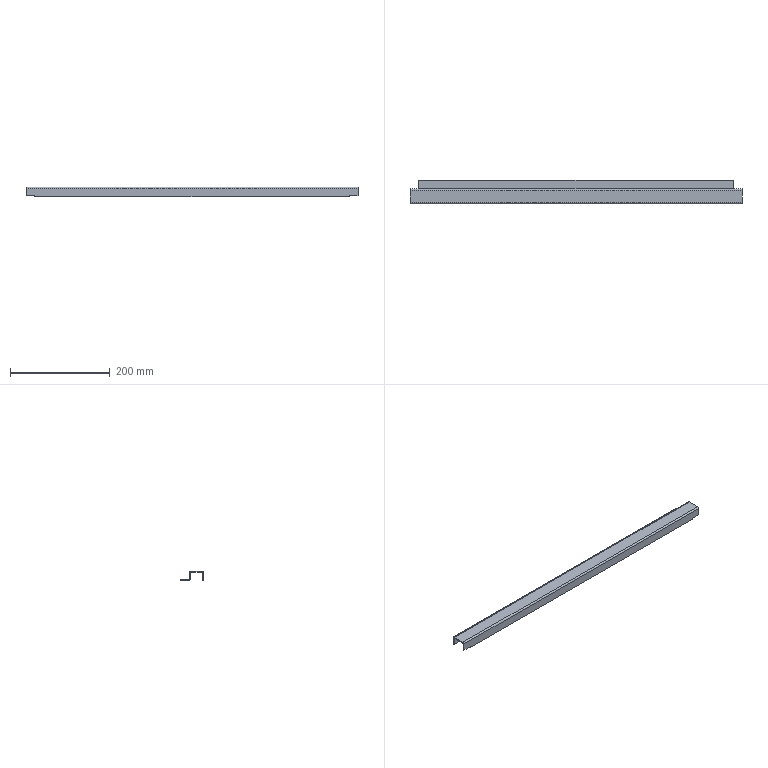Part | SolidWorks | features BaseBody 1 | 1 solid | 44 faces | box 667 x 48 x 20 mm | volume 107090 mm3 | plane 38 | cylinder 6 | commonest cylinder face diameters 2 x3 6 x3
STEP:
#1=CARTESIAN_POINT('',(-315.5,-13.,-18.));
#2=VERTEX_POINT('',#1);
#3=CARTESIAN_POINT('',(-315.5,-13.,-20.));
#4=VERTEX_POINT('',#3);
#5=CARTESIAN_POINT('',(-315.5,-13.,0.));
#6=DIRECTION('',(0.,0.,-1.));
#7=VECTOR('',#6,1000.);
#8=LINE('',#5,#7);
#9=EDGE_CURVE('',#2,#4,#8,.T.);
#10=ORIENTED_EDGE('',*,*,#9,.T.);
#11=CARTESIAN_POINT('',(-315.5,-15.,-20.));
#12=VERTEX_POINT('',#11);
#13=CARTESIAN_POINT('',(-315.5,33.,-20.));
#14=DIRECTION('',(0.,-1.,0.));
#15=VECTOR('',#14,1000.);
#16=LINE('',#13,#15);
#17=EDGE_CURVE('',#4,#12,#16,.T.);
#18=ORIENTED_EDGE('',*,*,#17,.T.);
#19=CARTESIAN_POINT('',(-315.5,-15.,-18.));
#20=VERTEX_POINT('',#19);
#21=CARTESIAN_POINT('',(-315.5,-15.,-20.));
#22=DIRECTION('',(0.,0.,1.));
#23=VECTOR('',#22,1000.);
#24=LINE('',#21,#23);
#25=EDGE_CURVE('',#12,#20,#24,.T.);
#26=ORIENTED_EDGE('',*,*,#25,.T.);
#27=CARTESIAN_POINT('',(-315.5,33.,-18.));
#28=DIRECTION('',(0.,-1.,0.));
#29=VECTOR('',#28,1000.);
#30=LINE('',#27,#29);
#31=EDGE_CURVE('',#2,#20,#30,.T.);
#32=ORIENTED_EDGE('',*,*,#31,.F.);
#33=EDGE_LOOP('',(#10,#18,#26,#32));
#34=FACE_OUTER_BOUND('',#33,.T.);
#35=CARTESIAN_POINT('',(-315.5,33.,-20.));
#36=DIRECTION('',(1.,0.,0.));
#37=DIRECTION('',(0.,1.,0.));
#38=AXIS2_PLACEMENT_3D('',#35,#36,#37);
#39=PLANE('',#38);
#40=ADVANCED_FACE('',(#34),#39,.F.);
#41=CARTESIAN_POINT('',(-333.5,-13.,-18.));
#42=VERTEX_POINT('',#41);
#43=CARTESIAN_POINT('',(0.,-13.,-18.));
#44=DIRECTION('',(1.,0.,0.));
#45=VECTOR('',#44,1000.);
#46=LINE('',#43,#45);
#47=EDGE_CURVE('',#42,#2,#46,.T.);
#48=ORIENTED_EDGE('',*,*,#47,.T.);
#49=ORIENTED_EDGE('',*,*,#31,.T.);
#50=CARTESIAN_POINT('',(-333.5,-15.,-18.));
#51=VERTEX_POINT('',#50);
#52=CARTESIAN_POINT('',(-333.5,-15.,-18.));
#53=DIRECTION('',(-1.,0.,0.));
#54=VECTOR('',#53,1000.);
#55=LINE('',#52,#54);
#56=EDGE_CURVE('',#20,#51,#55,.T.);
#57=ORIENTED_EDGE('',*,*,#56,.T.);
#58=CARTESIAN_POINT('',(-333.5,33.,-18.));
#59=DIRECTION('',(0.,-1.,0.));
#60=VECTOR('',#59,1000.);
#61=LINE('',#58,#60);
#62=EDGE_CURVE('',#42,#51,#61,.T.);
#63=ORIENTED_EDGE('',*,*,#62,.F.);
#64=EDGE_LOOP('',(#48,#49,#57,#63));
#65=FACE_OUTER_BOUND('',#64,.T.);
#66=CARTESIAN_POINT('',(-333.5,33.,-18.));
#67=DIRECTION('',(0.,0.,1.));
#68=DIRECTION('',(0.,-1.,0.));
#69=AXIS2_PLACEMENT_3D('',#66,#67,#68);
#70=PLANE('',#69);
#71=ADVANCED_FACE('',(#65),#70,.F.);
#72=CARTESIAN_POINT('',(315.5,-13.,-20.));
#73=VERTEX_POINT('',#72);
#74=CARTESIAN_POINT('',(315.5,-13.,-18.));
#75=VERTEX_POINT('',#74);
#76=CARTESIAN_POINT('',(315.5,-13.,0.));
#77=DIRECTION('',(0.,0.,1.));
#78=VECTOR('',#77,1000.);
#79=LINE('',#76,#78);
#80=EDGE_CURVE('',#73,#75,#79,.T.);
#81=ORIENTED_EDGE('',*,*,#80,.T.);
#82=CARTESIAN_POINT('',(315.5,-15.,-18.));
#83=VERTEX_POINT('',#82);
#84=CARTESIAN_POINT('',(315.5,33.,-18.));
#85=DIRECTION('',(0.,-1.,0.));
#86=VECTOR('',#85,1000.);
#87=LINE('',#84,#86);
#88=EDGE_CURVE('',#75,#83,#87,.T.);
#89=ORIENTED_EDGE('',*,*,#88,.T.);
#90=CARTESIAN_POINT('',(315.5,-15.,-20.));
#91=VERTEX_POINT('',#90);
#92=CARTESIAN_POINT('',(315.5,-15.,-20.));
#93=DIRECTION('',(0.,0.,-1.));
#94=VECTOR('',#93,1000.);
#95=LINE('',#92,#94);
#96=EDGE_CURVE('',#83,#91,#95,.T.);
#97=ORIENTED_EDGE('',*,*,#96,.T.);
#98=CARTESIAN_POINT('',(315.5,33.,-20.));
#99=DIRECTION('',(0.,-1.,0.));
#100=VECTOR('',#99,1000.);
#101=LINE('',#98,#100);
#102=EDGE_CURVE('',#73,#91,#101,.T.);
#103=ORIENTED_EDGE('',*,*,#102,.F.);
#104=EDGE_LOOP('',(#81,#89,#97,#103));
#105=FACE_OUTER_BOUND('',#104,.T.);
#106=CARTESIAN_POINT('',(315.5,33.,-20.));
#107=DIRECTION('',(-1.,0.,0.));
#108=DIRECTION('',(0.,1.,0.));
#109=AXIS2_PLACEMENT_3D('',#106,#107,#108);
#110=PLANE('',#109);
#111=ADVANCED_FACE('',(#105),#110,.F.);
#112=CARTESIAN_POINT('',(333.5,-13.,-18.));
#113=VERTEX_POINT('',#112);
#114=CARTESIAN_POINT('',(0.,-13.,-18.));
#115=DIRECTION('',(1.,0.,0.));
#116=VECTOR('',#115,1000.);
#117=LINE('',#114,#116);
#118=EDGE_CURVE('',#75,#113,#117,.T.);
#119=ORIENTED_EDGE('',*,*,#118,.T.);
#120=CARTESIAN_POINT('',(333.5,-15.,-18.));
#121=VERTEX_POINT('',#120);
#122=CARTESIAN_POINT('',(333.5,33.,-18.));
#123=DIRECTION('',(0.,-1.,0.));
#124=VECTOR('',#123,1000.);
#125=LINE('',#122,#124);
#126=EDGE_CURVE('',#113,#121,#125,.T.);
#127=ORIENTED_EDGE('',*,*,#126,.T.);
#128=CARTESIAN_POINT('',(333.5,-15.,-18.));
#129=DIRECTION('',(-1.,0.,0.));
#130=VECTOR('',#129,1000.);
#131=LINE('',#128,#130);
#132=EDGE_CURVE('',#121,#83,#131,.T.);
#133=ORIENTED_EDGE('',*,*,#132,.T.);
#134=ORIENTED_EDGE('',*,*,#88,.F.);
#135=EDGE_LOOP('',(#119,#127,#133,#134));
#136=FACE_OUTER_BOUND('',#135,.T.);
#137=CARTESIAN_POINT('',(333.5,33.,-18.));
#138=DIRECTION('',(0.,0.,1.));
#139=DIRECTION('',(0.,-1.,0.));
#140=AXIS2_PLACEMENT_3D('',#137,#138,#139);
#141=PLANE('',#140);
#142=ADVANCED_FACE('',(#136),#141,.F.);
#143=CARTESIAN_POINT('',(-333.5,15.,-18.));
#144=VERTEX_POINT('',#143);
#145=CARTESIAN_POINT('',(-316.5,15.,-18.));
#146=VERTEX_POINT('',#145);
#147=CARTESIAN_POINT('',(0.,15.,-18.));
#148=DIRECTION('',(1.,0.,0.));
#149=VECTOR('',#148,1000.);
#150=LINE('',#147,#149);
#151=EDGE_CURVE('',#144,#146,#150,.T.);
#152=ORIENTED_EDGE('',*,*,#151,.T.);
#153=CARTESIAN_POINT('',(-316.5,13.,-18.));
#154=VERTEX_POINT('',#153);
#155=CARTESIAN_POINT('',(-316.5,15.,-18.));
#156=DIRECTION('',(0.,-1.,0.));
#157=VECTOR('',#156,1000.);
#158=LINE('',#155,#157);
#159=EDGE_CURVE('',#146,#154,#158,.T.);
#160=ORIENTED_EDGE('',*,*,#159,.T.);
#161=CARTESIAN_POINT('',(-333.5,13.,-18.));
#162=VERTEX_POINT('',#161);
#163=CARTESIAN_POINT('',(0.,13.,-18.));
#164=DIRECTION('',(1.,0.,0.));
#165=VECTOR('',#164,1000.);
#166=LINE('',#163,#165);
#167=EDGE_CURVE('',#162,#154,#166,.T.);
#168=ORIENTED_EDGE('',*,*,#167,.F.);
#169=CARTESIAN_POINT('',(-333.5,33.,-18.));
#170=DIRECTION('',(0.,-1.,0.));
#171=VECTOR('',#170,1000.);
#172=LINE('',#169,#171);
#173=EDGE_CURVE('',#144,#162,#172,.T.);
#174=ORIENTED_EDGE('',*,*,#173,.F.);
#175=EDGE_LOOP('',(#152,#160,#168,#174));
#176=FACE_OUTER_BOUND('',#175,.T.);
#177=CARTESIAN_POINT('',(-333.5,33.,-18.));
#178=DIRECTION('',(0.,0.,1.));
#179=DIRECTION('',(0.,-1.,0.));
#180=AXIS2_PLACEMENT_3D('',#177,#178,#179);
#181=PLANE('',#180);
#182=ADVANCED_FACE('',(#176),#181,.F.);
#183=CARTESIAN_POINT('',(316.5,15.,-18.));
#184=VERTEX_POINT('',#183);
#185=CARTESIAN_POINT('',(333.5,15.,-18.));
#186=VERTEX_POINT('',#185);
#187=CARTESIAN_POINT('',(0.,15.,-18.));
#188=DIRECTION('',(1.,0.,0.));
#189=VECTOR('',#188,1000.);
#190=LINE('',#187,#189);
#191=EDGE_CURVE('',#184,#186,#190,.T.);
#192=ORIENTED_EDGE('',*,*,#191,.T.);
#193=CARTESIAN_POINT('',(333.5,13.,-18.));
#194=VERTEX_POINT('',#193);
#195=CARTESIAN_POINT('',(333.5,33.,-18.));
#196=DIRECTION('',(0.,-1.,0.));
#197=VECTOR('',#196,1000.);
#198=LINE('',#195,#197);
#199=EDGE_CURVE('',#186,#194,#198,.T.);
#200=ORIENTED_EDGE('',*,*,#199,.T.);
#201=CARTESIAN_POINT('',(316.5,13.,-18.));
#202=VERTEX_POINT('',#201);
#203=CARTESIAN_POINT('',(0.,13.,-18.));
#204=DIRECTION('',(1.,0.,0.));
#205=VECTOR('',#204,1000.);
#206=LINE('',#203,#205);
#207=EDGE_CURVE('',#202,#194,#206,.T.);
#208=ORIENTED_EDGE('',*,*,#207,.F.);
#209=CARTESIAN_POINT('',(316.5,15.,-18.));
#210=DIRECTION('',(0.,1.,0.));
#211=VECTOR('',#210,1000.);
#212=LINE('',#209,#211);
#213=EDGE_CURVE('',#202,#184,#212,.T.);
#214=ORIENTED_EDGE('',*,*,#213,.T.);
#215=EDGE_LOOP('',(#192,#200,#208,#214));
#216=FACE_OUTER_BOUND('',#215,.T.);
#217=CARTESIAN_POINT('',(333.5,33.,-18.));
#218=DIRECTION('',(0.,0.,1.));
#219=DIRECTION('',(0.,-1.,0.));
#220=AXIS2_PLACEMENT_3D('',#217,#218,#219);
#221=PLANE('',#220);
#222=ADVANCED_FACE('',(#216),#221,.F.);
#223=CARTESIAN_POINT('',(315.5,33.,-18.));
#224=VERTEX_POINT('',#223);
#225=CARTESIAN_POINT('',(-315.5,33.,-18.));
#226=VERTEX_POINT('',#225);
#227=CARTESIAN_POINT('',(0.,33.,-18.));
#228=DIRECTION('',(-1.,0.,0.));
#229=VECTOR('',#228,1000.);
#230=LINE('',#227,#229);
#231=EDGE_CURVE('',#224,#226,#230,.T.);
#232=ORIENTED_EDGE('',*,*,#231,.F.);
#233=CARTESIAN_POINT('',(315.5,33.,-20.));
#234=VERTEX_POINT('',#233);
#235=CARTESIAN_POINT('',(315.5,33.,-20.));
#236=DIRECTION('',(0.,0.,1.));
#237=VECTOR('',#236,1000.);
#238=LINE('',#235,#237);
#239=EDGE_CURVE('',#234,#224,#238,.T.);
#240=ORIENTED_EDGE('',*,*,#239,.F.);
#241=CARTESIAN_POINT('',(-315.5,33.,-20.));
#242=VERTEX_POINT('',#241);
#243=CARTESIAN_POINT('',(-315.5,33.,-20.));
#244=DIRECTION('',(-1.,0.,0.));
#245=VECTOR('',#244,1000.);
#246=LINE('',#243,#245);
#247=EDGE_CURVE('',#234,#242,#246,.T.);
#248=ORIENTED_EDGE('',*,*,#247,.T.);
#249=CARTESIAN_POINT('',(-315.5,33.,-20.));
#250=DIRECTION('',(0.,0.,1.));
#251=VECTOR('',#250,1000.);
#252=LINE('',#249,#251);
#253=EDGE_CURVE('',#242,#226,#252,.T.);
#254=ORIENTED_EDGE('',*,*,#253,.T.);
#255=EDGE_LOOP('',(#232,#240,#248,#254));
#256=FACE_OUTER_BOUND('',#255,.T.);
#257=CARTESIAN_POINT('',(-315.5,33.,-20.));
#258=DIRECTION('',(0.,1.,0.));
#259=DIRECTION('',(1.,0.,0.));
#260=AXIS2_PLACEMENT_3D('',#257,#258,#259);
#261=PLANE('',#260);
#262=ADVANCED_FACE('',(#256),#261,.T.);
#263=CARTESIAN_POINT('',(315.5,16.,-18.));
#264=VERTEX_POINT('',#263);
#265=CARTESIAN_POINT('',(-315.5,16.,-18.));
#266=VERTEX_POINT('',#265);
#267=CARTESIAN_POINT('',(315.5,16.,-18.));
#268=DIRECTION('',(-1.,0.,0.));
#269=VECTOR('',#268,1000.);
#270=LINE('',#267,#269);
#271=EDGE_CURVE('',#264,#266,#270,.T.);
#272=ORIENTED_EDGE('',*,*,#271,.F.);
#273=CARTESIAN_POINT('',(315.5,0.,-18.));
#274=DIRECTION('',(0.,1.,0.));
#275=VECTOR('',#274,1000.);
#276=LINE('',#273,#275);
#277=EDGE_CURVE('',#264,#224,#276,.T.);
#278=ORIENTED_EDGE('',*,*,#277,.T.);
#279=ORIENTED_EDGE('',*,*,#231,.T.);
#280=CARTESIAN_POINT('',(-315.5,0.,-18.));
#281=DIRECTION('',(0.,-1.,0.));
#282=VECTOR('',#281,1000.);
#283=LINE('',#280,#282);
#284=EDGE_CURVE('',#226,#266,#283,.T.);
#285=ORIENTED_EDGE('',*,*,#284,.T.);
#286=EDGE_LOOP('',(#272,#278,#279,#285));
#287=FACE_OUTER_BOUND('',#286,.T.);
#288=CARTESIAN_POINT('',(0.,0.,-18.));
#289=DIRECTION('',(0.,0.,-1.));
#290=DIRECTION('',(0.,-1.,0.));
#291=AXIS2_PLACEMENT_3D('',#288,#289,#290);
#292=PLANE('',#291);
#293=ADVANCED_FACE('',(#287),#292,.F.);
#294=CARTESIAN_POINT('',(315.5,16.,-20.));
#295=VERTEX_POINT('',#294);
#296=CARTESIAN_POINT('',(315.5,15.,-20.));
#297=DIRECTION('',(0.,1.,0.));
#298=VECTOR('',#297,1000.);
#299=LINE('',#296,#298);
#300=EDGE_CURVE('',#295,#234,#299,.T.);
#301=ORIENTED_EDGE('',*,*,#300,.F.);
#302=CARTESIAN_POINT('',(-315.5,16.,-20.));
#303=VERTEX_POINT('',#302);
#304=CARTESIAN_POINT('',(0.,16.,-20.));
#305=DIRECTION('',(-1.,0.,0.));
#306=VECTOR('',#305,1000.);
#307=LINE('',#304,#306);
#308=EDGE_CURVE('',#295,#303,#307,.T.);
#309=ORIENTED_EDGE('',*,*,#308,.T.);
#310=CARTESIAN_POINT('',(-315.5,15.,-20.));
#311=DIRECTION('',(0.,-1.,0.));
#312=VECTOR('',#311,1000.);
#313=LINE('',#310,#312);
#314=EDGE_CURVE('',#242,#303,#313,.T.);
#315=ORIENTED_EDGE('',*,*,#314,.F.);
#316=ORIENTED_EDGE('',*,*,#247,.F.);
#317=EDGE_LOOP('',(#301,#309,#315,#316));
#318=FACE_OUTER_BOUND('',#317,.T.);
#319=CARTESIAN_POINT('',(0.,0.,-20.));
#320=DIRECTION('',(0.,0.,-1.));
#321=DIRECTION('',(0.,-1.,0.));
#322=AXIS2_PLACEMENT_3D('',#319,#320,#321);
#323=PLANE('',#322);
#324=ADVANCED_FACE('',(#318),#323,.T.);
#325=ORIENTED_EDGE('',*,*,#314,.T.);
#326=CARTESIAN_POINT('',(-315.5,16.,-18.));
#327=DIRECTION('',(0.,0.,-1.));
#328=VECTOR('',#327,1000.);
#329=LINE('',#326,#328);
#330=EDGE_CURVE('',#266,#303,#329,.T.);
#331=ORIENTED_EDGE('',*,*,#330,.F.);
#332=ORIENTED_EDGE('',*,*,#284,.F.);
#333=ORIENTED_EDGE('',*,*,#253,.F.);
#334=EDGE_LOOP('',(#325,#331,#332,#333));
#335=FACE_OUTER_BOUND('',#334,.T.);
#336=CARTESIAN_POINT('',(-315.5,15.,-20.));
#337=DIRECTION('',(-1.,0.,0.));
#338=DIRECTION('',(0.,0.,1.));
#339=AXIS2_PLACEMENT_3D('',#336,#337,#338);
#340=PLANE('',#339);
#341=ADVANCED_FACE('',(#335),#340,.T.);
#342=ORIENTED_EDGE('',*,*,#277,.F.);
#343=CARTESIAN_POINT('',(315.5,16.,-20.));
#344=DIRECTION('',(0.,0.,-1.));
#345=VECTOR('',#344,1000.);
#346=LINE('',#343,#345);
#347=EDGE_CURVE('',#264,#295,#346,.T.);
#348=ORIENTED_EDGE('',*,*,#347,.T.);
#349=ORIENTED_EDGE('',*,*,#300,.T.);
#350=ORIENTED_EDGE('',*,*,#239,.T.);
#351=EDGE_LOOP('',(#342,#348,#349,#350));
#352=FACE_OUTER_BOUND('',#351,.T.);
#353=CARTESIAN_POINT('',(315.5,15.,-20.));
#354=DIRECTION('',(1.,0.,0.));
#355=DIRECTION('',(0.,1.,0.));
#356=AXIS2_PLACEMENT_3D('',#353,#354,#355);
#357=PLANE('',#356);
#358=ADVANCED_FACE('',(#352),#357,.T.);
#359=CARTESIAN_POINT('',(-315.5,15.,-17.));
#360=VERTEX_POINT('',#359);
#361=CARTESIAN_POINT('',(315.5,15.,-17.));
#362=VERTEX_POINT('',#361);
#363=CARTESIAN_POINT('',(-315.5,15.,-17.));
#364=DIRECTION('',(1.,0.,0.));
#365=VECTOR('',#364,1000.);
#366=LINE('',#363,#365);
#367=EDGE_CURVE('',#360,#362,#366,.T.);
#368=ORIENTED_EDGE('',*,*,#367,.T.);
#369=CARTESIAN_POINT('',(315.5,16.,-17.));
#370=DIRECTION('',(1.,0.,0.));
#371=DIRECTION('',(0.,0.,1.));
#372=AXIS2_PLACEMENT_3D('',#369,#370,#371);
#373=CIRCLE('',#372,1.);
#374=EDGE_CURVE('',#362,#264,#373,.T.);
#375=ORIENTED_EDGE('',*,*,#374,.T.);
#376=ORIENTED_EDGE('',*,*,#271,.T.);
#377=CARTESIAN_POINT('',(-315.5,16.,-17.));
#378=DIRECTION('',(-1.,0.,0.));
#379=DIRECTION('',(0.,0.,1.));
#380=AXIS2_PLACEMENT_3D('',#377,#378,#379);
#381=CIRCLE('',#380,1.);
#382=EDGE_CURVE('',#266,#360,#381,.T.);
#383=ORIENTED_EDGE('',*,*,#382,.T.);
#384=EDGE_LOOP('',(#368,#375,#376,#383));
#385=FACE_OUTER_BOUND('',#384,.T.);
#386=CARTESIAN_POINT('',(-315.5,16.,-17.));
#387=DIRECTION('',(-1.,0.,0.));
#388=DIRECTION('',(0.,0.,-1.));
#389=AXIS2_PLACEMENT_3D('',#386,#387,#388);
#390=CYLINDRICAL_SURFACE('',#389,1.);
#391=ADVANCED_FACE('',(#385),#390,.F.);
#392=CARTESIAN_POINT('',(-315.5,13.,-17.));
#393=VERTEX_POINT('',#392);
#394=CARTESIAN_POINT('',(315.5,13.,-17.));
#395=VERTEX_POINT('',#394);
#396=CARTESIAN_POINT('',(-315.5,13.,-17.));
#397=DIRECTION('',(1.,0.,0.));
#398=VECTOR('',#397,1000.);
#399=LINE('',#396,#398);
#400=EDGE_CURVE('',#393,#395,#399,.T.);
#401=ORIENTED_EDGE('',*,*,#400,.F.);
#402=CARTESIAN_POINT('',(-315.5,13.172,-18.));
#403=VERTEX_POINT('',#402);
#404=CARTESIAN_POINT('',(-315.5,16.,-17.));
#405=DIRECTION('',(-1.,0.,0.));
#406=DIRECTION('',(0.,0.,1.));
#407=AXIS2_PLACEMENT_3D('',#404,#405,#406);
#408=CIRCLE('',#407,3.);
#409=EDGE_CURVE('',#403,#393,#408,.T.);
#410=ORIENTED_EDGE('',*,*,#409,.F.);
#411=CARTESIAN_POINT('',(-315.5,16.,-17.));
#412=DIRECTION('',(-1.,0.,0.));
#413=DIRECTION('',(0.,0.,1.));
#414=AXIS2_PLACEMENT_3D('',#411,#412,#413);
#415=CIRCLE('',#414,3.);
#416=EDGE_CURVE('',#303,#403,#415,.T.);
#417=ORIENTED_EDGE('',*,*,#416,.F.);
#418=ORIENTED_EDGE('',*,*,#308,.F.);
#419=CARTESIAN_POINT('',(315.5,13.172,-18.));
#420=VERTEX_POINT('',#419);
#421=CARTESIAN_POINT('',(315.5,16.,-17.));
#422=DIRECTION('',(1.,0.,0.));
#423=DIRECTION('',(0.,0.,1.));
#424=AXIS2_PLACEMENT_3D('',#421,#422,#423);
#425=CIRCLE('',#424,3.);
#426=EDGE_CURVE('',#420,#295,#425,.T.);
#427=ORIENTED_EDGE('',*,*,#426,.F.);
#428=CARTESIAN_POINT('',(315.5,16.,-17.));
#429=DIRECTION('',(1.,0.,0.));
#430=DIRECTION('',(0.,0.,1.));
#431=AXIS2_PLACEMENT_3D('',#428,#429,#430);
#432=CIRCLE('',#431,3.);
#433=EDGE_CURVE('',#395,#420,#432,.T.);
#434=ORIENTED_EDGE('',*,*,#433,.F.);
#435=EDGE_LOOP('',(#401,#410,#417,#418,#427,#434));
#436=FACE_OUTER_BOUND('',#435,.T.);
#437=CARTESIAN_POINT('',(-315.5,16.,-17.));
#438=DIRECTION('',(-1.,0.,0.));
#439=DIRECTION('',(0.,0.,-1.));
#440=AXIS2_PLACEMENT_3D('',#437,#438,#439);
#441=CYLINDRICAL_SURFACE('',#440,3.);
#442=ADVANCED_FACE('',(#436),#441,.T.);
#443=CARTESIAN_POINT('',(-315.5,16.,-18.));
#444=DIRECTION('',(0.,1.,0.));
#445=VECTOR('',#444,1000.);
#446=LINE('',#443,#445);
#447=EDGE_CURVE('',#403,#266,#446,.T.);
#448=ORIENTED_EDGE('',*,*,#447,.F.);
#449=ORIENTED_EDGE('',*,*,#409,.T.);
#450=CARTESIAN_POINT('',(-315.5,15.,-17.));
#451=DIRECTION('',(0.,-1.,0.));
#452=VECTOR('',#451,1000.);
#453=LINE('',#450,#452);
#454=EDGE_CURVE('',#360,#393,#453,.T.);
#455=ORIENTED_EDGE('',*,*,#454,.F.);
#456=ORIENTED_EDGE('',*,*,#382,.F.);
#457=EDGE_LOOP('',(#448,#449,#455,#456));
#458=FACE_OUTER_BOUND('',#457,.T.);
#459=CARTESIAN_POINT('',(-315.5,16.,-17.));
#460=DIRECTION('',(1.,0.,0.));
#461=DIRECTION('',(0.,1.,0.));
#462=AXIS2_PLACEMENT_3D('',#459,#460,#461);
#463=PLANE('',#462);
#464=ADVANCED_FACE('',(#458),#463,.F.);
#465=CARTESIAN_POINT('',(315.5,16.,-18.));
#466=DIRECTION('',(0.,-1.,0.));
#467=VECTOR('',#466,1000.);
#468=LINE('',#465,#467);
#469=EDGE_CURVE('',#264,#420,#468,.T.);
#470=ORIENTED_EDGE('',*,*,#469,.F.);
#471=ORIENTED_EDGE('',*,*,#374,.F.);
#472=CARTESIAN_POINT('',(315.5,15.,-17.));
#473=DIRECTION('',(0.,-1.,0.));
#474=VECTOR('',#473,1000.);
#475=LINE('',#472,#474);
#476=EDGE_CURVE('',#362,#395,#475,.T.);
#477=ORIENTED_EDGE('',*,*,#476,.T.);
#478=ORIENTED_EDGE('',*,*,#433,.T.);
#479=EDGE_LOOP('',(#470,#471,#477,#478));
#480=FACE_OUTER_BOUND('',#479,.T.);
#481=CARTESIAN_POINT('',(315.5,16.,-17.));
#482=DIRECTION('',(1.,0.,0.));
#483=DIRECTION('',(0.,1.,0.));
#484=AXIS2_PLACEMENT_3D('',#481,#482,#483);
#485=PLANE('',#484);
#486=ADVANCED_FACE('',(#480),#485,.T.);
#487=ORIENTED_EDGE('',*,*,#213,.F.);
#488=CARTESIAN_POINT('',(316.5,13.,-16.));
#489=VERTEX_POINT('',#488);
#490=CARTESIAN_POINT('',(316.5,13.,0.));
#491=DIRECTION('',(0.,0.,1.));
#492=VECTOR('',#491,1000.);
#493=LINE('',#490,#492);
#494=EDGE_CURVE('',#202,#489,#493,.T.);
#495=ORIENTED_EDGE('',*,*,#494,.T.);
#496=CARTESIAN_POINT('',(316.5,15.,-16.));
#497=VERTEX_POINT('',#496);
#498=CARTESIAN_POINT('',(316.5,15.,-16.));
#499=DIRECTION('',(0.,-1.,0.));
#500=VECTOR('',#499,1000.);
#501=LINE('',#498,#500);
#502=EDGE_CURVE('',#497,#489,#501,.T.);
#503=ORIENTED_EDGE('',*,*,#502,.F.);
#504=CARTESIAN_POINT('',(316.5,15.,-16.));
#505=DIRECTION('',(0.,0.,-1.));
#506=VECTOR('',#505,1000.);
#507=LINE('',#504,#506);
#508=EDGE_CURVE('',#497,#184,#507,.T.);
#509=ORIENTED_EDGE('',*,*,#508,.T.);
#510=EDGE_LOOP('',(#487,#495,#503,#509));
#511=FACE_OUTER_BOUND('',#510,.T.);
#512=CARTESIAN_POINT('',(316.5,15.,-16.));
#513=DIRECTION('',(-1.,0.,0.));
#514=DIRECTION('',(0.,0.,1.));
#515=AXIS2_PLACEMENT_3D('',#512,#513,#514);
#516=PLANE('',#515);
#517=ADVANCED_FACE('',(#511),#516,.T.);
#518=ORIENTED_EDGE('',*,*,#159,.F.);
#519=CARTESIAN_POINT('',(-316.5,15.,-16.));
#520=VERTEX_POINT('',#519);
#521=CARTESIAN_POINT('',(-316.5,15.,-20.));
#522=DIRECTION('',(0.,0.,1.));
#523=VECTOR('',#522,1000.);
#524=LINE('',#521,#523);
#525=EDGE_CURVE('',#146,#520,#524,.T.);
#526=ORIENTED_EDGE('',*,*,#525,.T.);
#527=CARTESIAN_POINT('',(-316.5,13.,-16.));
#528=VERTEX_POINT('',#527);
#529=CARTESIAN_POINT('',(-316.5,15.,-16.));
#530=DIRECTION('',(0.,-1.,0.));
#531=VECTOR('',#530,1000.);
#532=LINE('',#529,#531);
#533=EDGE_CURVE('',#520,#528,#532,.T.);
#534=ORIENTED_EDGE('',*,*,#533,.T.);
#535=CARTESIAN_POINT('',(-316.5,13.,0.));
#536=DIRECTION('',(0.,0.,-1.));
#537=VECTOR('',#536,1000.);
#538=LINE('',#535,#537);
#539=EDGE_CURVE('',#528,#154,#538,.T.);
#540=ORIENTED_EDGE('',*,*,#539,.T.);
#541=EDGE_LOOP('',(#518,#526,#534,#540));
#542=FACE_OUTER_BOUND('',#541,.T.);
#543=CARTESIAN_POINT('',(-316.5,15.,-20.));
#544=DIRECTION('',(1.,0.,0.));
#545=DIRECTION('',(0.,1.,0.));
#546=AXIS2_PLACEMENT_3D('',#543,#544,#545);
#547=PLANE('',#546);
#548=ADVANCED_FACE('',(#542),#547,.T.);
#549=ORIENTED_EDGE('',*,*,#502,.T.);
#550=CARTESIAN_POINT('',(315.5,13.,-16.));
#551=VERTEX_POINT('',#550);
#552=CARTESIAN_POINT('',(0.,13.,-16.));
#553=DIRECTION('',(-1.,0.,0.));
#554=VECTOR('',#553,1000.);
#555=LINE('',#552,#554);
#556=EDGE_CURVE('',#489,#551,#555,.T.);
#557=ORIENTED_EDGE('',*,*,#556,.T.);
#558=CARTESIAN_POINT('',(315.5,15.,-16.));
#559=VERTEX_POINT('',#558);
#560=CARTESIAN_POINT('',(315.5,15.,-16.));
#561=DIRECTION('',(0.,-1.,0.));
#562=VECTOR('',#561,1000.);
#563=LINE('',#560,#562);
#564=EDGE_CURVE('',#559,#551,#563,.T.);
#565=ORIENTED_EDGE('',*,*,#564,.F.);
#566=CARTESIAN_POINT('',(315.5,15.,-16.));
#567=DIRECTION('',(1.,0.,0.));
#568=VECTOR('',#567,1000.);
#569=LINE('',#566,#568);
#570=EDGE_CURVE('',#559,#497,#569,.T.);
#571=ORIENTED_EDGE('',*,*,#570,.T.);
#572=EDGE_LOOP('',(#549,#557,#565,#571));
#573=FACE_OUTER_BOUND('',#572,.T.);
#574=CARTESIAN_POINT('',(315.5,15.,-16.));
#575=DIRECTION('',(0.,0.,-1.));
#576=DIRECTION('',(-1.,0.,0.));
#577=AXIS2_PLACEMENT_3D('',#574,#575,#576);
#578=PLANE('',#577);
#579=ADVANCED_FACE('',(#573),#578,.T.);
#580=ORIENTED_EDGE('',*,*,#564,.T.);
#581=CARTESIAN_POINT('',(315.5,13.,0.));
#582=DIRECTION('',(0.,0.,-1.));
#583=VECTOR('',#582,1000.);
#584=LINE('',#581,#583);
#585=EDGE_CURVE('',#551,#395,#584,.T.);
#586=ORIENTED_EDGE('',*,*,#585,.T.);
#587=ORIENTED_EDGE('',*,*,#476,.F.);
#588=CARTESIAN_POINT('',(315.5,15.,-17.));
#589=DIRECTION('',(0.,0.,1.));
#590=VECTOR('',#589,1000.);
#591=LINE('',#588,#590);
#592=EDGE_CURVE('',#362,#559,#591,.T.);
#593=ORIENTED_EDGE('',*,*,#592,.T.);
#594=EDGE_LOOP('',(#580,#586,#587,#593));
#595=FACE_OUTER_BOUND('',#594,.T.);
#596=CARTESIAN_POINT('',(315.5,15.,-17.));
#597=DIRECTION('',(1.,0.,0.));
#598=DIRECTION('',(0.,1.,0.));
#599=AXIS2_PLACEMENT_3D('',#596,#597,#598);
#600=PLANE('',#599);
#601=ADVANCED_FACE('',(#595),#600,.T.);
#602=ORIENTED_EDGE('',*,*,#454,.T.);
#603=CARTESIAN_POINT('',(-315.5,13.,-16.));
#604=VERTEX_POINT('',#603);
#605=CARTESIAN_POINT('',(-315.5,13.,0.));
#606=DIRECTION('',(0.,0.,1.));
#607=VECTOR('',#606,1000.);
#608=LINE('',#605,#607);
#609=EDGE_CURVE('',#393,#604,#608,.T.);
#610=ORIENTED_EDGE('',*,*,#609,.T.);
#611=CARTESIAN_POINT('',(-315.5,15.,-16.));
#612=VERTEX_POINT('',#611);
#613=CARTESIAN_POINT('',(-315.5,15.,-16.));
#614=DIRECTION('',(0.,-1.,0.));
#615=VECTOR('',#614,1000.);
#616=LINE('',#613,#615);
#617=EDGE_CURVE('',#612,#604,#616,.T.);
#618=ORIENTED_EDGE('',*,*,#617,.F.);
#619=CARTESIAN_POINT('',(-315.5,15.,-16.));
#620=DIRECTION('',(0.,0.,-1.));
#621=VECTOR('',#620,1000.);
#622=LINE('',#619,#621);
#623=EDGE_CURVE('',#612,#360,#622,.T.);
#624=ORIENTED_EDGE('',*,*,#623,.T.);
#625=EDGE_LOOP('',(#602,#610,#618,#624));
#626=FACE_OUTER_BOUND('',#625,.T.);
#627=CARTESIAN_POINT('',(-315.5,15.,-16.));
#628=DIRECTION('',(-1.,0.,0.));
#629=DIRECTION('',(0.,0.,1.));
#630=AXIS2_PLACEMENT_3D('',#627,#628,#629);
#631=PLANE('',#630);
#632=ADVANCED_FACE('',(#626),#631,.T.);
#633=ORIENTED_EDGE('',*,*,#617,.T.);
#634=CARTESIAN_POINT('',(0.,13.,-16.));
#635=DIRECTION('',(-1.,0.,0.));
#636=VECTOR('',#635,1000.);
#637=LINE('',#634,#636);
#638=EDGE_CURVE('',#604,#528,#637,.T.);
#639=ORIENTED_EDGE('',*,*,#638,.T.);
#640=ORIENTED_EDGE('',*,*,#533,.F.);
#641=CARTESIAN_POINT('',(-316.5,15.,-16.));
#642=DIRECTION('',(1.,0.,0.));
#643=VECTOR('',#642,1000.);
#644=LINE('',#641,#643);
#645=EDGE_CURVE('',#520,#612,#644,.T.);
#646=ORIENTED_EDGE('',*,*,#645,.T.);
#647=EDGE_LOOP('',(#633,#639,#640,#646));
#648=FACE_OUTER_BOUND('',#647,.T.);
#649=CARTESIAN_POINT('',(-316.5,15.,-16.));
#650=DIRECTION('',(0.,0.,-1.));
#651=DIRECTION('',(-1.,0.,0.));
#652=AXIS2_PLACEMENT_3D('',#649,#650,#651);
#653=PLANE('',#652);
#654=ADVANCED_FACE('',(#648),#653,.T.);
#655=ORIENTED_EDGE('',*,*,#17,.F.);
#656=CARTESIAN_POINT('',(0.,-13.,-20.));
#657=DIRECTION('',(-1.,0.,0.));
#658=VECTOR('',#657,1000.);
#659=LINE('',#656,#658);
#660=EDGE_CURVE('',#73,#4,#659,.T.);
#661=ORIENTED_EDGE('',*,*,#660,.F.);
#662=ORIENTED_EDGE('',*,*,#102,.T.);
#663=CARTESIAN_POINT('',(333.5,-15.,-20.));
#664=DIRECTION('',(-1.,0.,0.));
#665=VECTOR('',#664,1000.);
#666=LINE('',#663,#665);
#667=EDGE_CURVE('',#91,#12,#666,.T.);
#668=ORIENTED_EDGE('',*,*,#667,.T.);
#669=EDGE_LOOP('',(#655,#661,#662,#668));
#670=FACE_OUTER_BOUND('',#669,.T.);
#671=CARTESIAN_POINT('',(333.5,-15.,-20.));
#672=DIRECTION('',(0.,0.,-1.));
#673=DIRECTION('',(0.,-1.,0.));
#674=AXIS2_PLACEMENT_3D('',#671,#672,#673);
#675=PLANE('',#674);
#676=ADVANCED_FACE('',(#670),#675,.T.);
#677=ORIENTED_EDGE('',*,*,#47,.F.);
#678=CARTESIAN_POINT('',(-333.5,-13.,-3.));
#679=VERTEX_POINT('',#678);
#680=CARTESIAN_POINT('',(-333.5,-13.,0.));
#681=DIRECTION('',(0.,0.,1.));
#682=VECTOR('',#681,1000.);
#683=LINE('',#680,#682);
#684=EDGE_CURVE('',#42,#679,#683,.T.);
#685=ORIENTED_EDGE('',*,*,#684,.T.);
#686=CARTESIAN_POINT('',(333.5,-13.,-3.));
#687=VERTEX_POINT('',#686);
#688=CARTESIAN_POINT('',(333.5,-13.,-3.));
#689=DIRECTION('',(-1.,0.,0.));
#690=VECTOR('',#689,1000.);
#691=LINE('',#688,#690);
#692=EDGE_CURVE('',#687,#679,#691,.T.);
#693=ORIENTED_EDGE('',*,*,#692,.F.);
#694=CARTESIAN_POINT('',(333.5,-13.,0.));
#695=DIRECTION('',(0.,0.,-1.));
#696=VECTOR('',#695,1000.);
#697=LINE('',#694,#696);
#698=EDGE_CURVE('',#687,#113,#697,.T.);
#699=ORIENTED_EDGE('',*,*,#698,.T.);
#700=ORIENTED_EDGE('',*,*,#118,.F.);
#701=ORIENTED_EDGE('',*,*,#80,.F.);
#702=ORIENTED_EDGE('',*,*,#660,.T.);
#703=ORIENTED_EDGE('',*,*,#9,.F.);
#704=EDGE_LOOP('',(#677,#685,#693,#699,#700,#701,#702,#703));
#705=FACE_OUTER_BOUND('',#704,.T.);
#706=CARTESIAN_POINT('',(0.,-13.,0.));
#707=DIRECTION('',(0.,1.,0.));
#708=DIRECTION('',(0.,0.,-1.));
#709=AXIS2_PLACEMENT_3D('',#706,#707,#708);
#710=PLANE('',#709);
#711=ADVANCED_FACE('',(#705),#710,.T.);
#712=CARTESIAN_POINT('',(-333.5,-15.,-3.));
#713=VERTEX_POINT('',#712);
#714=CARTESIAN_POINT('',(-333.5,-15.,-20.));
#715=DIRECTION('',(0.,0.,1.));
#716=VECTOR('',#715,1000.);
#717=LINE('',#714,#716);
#718=EDGE_CURVE('',#51,#713,#717,.T.);
#719=ORIENTED_EDGE('',*,*,#718,.F.);
#720=ORIENTED_EDGE('',*,*,#56,.F.);
#721=ORIENTED_EDGE('',*,*,#25,.F.);
#722=ORIENTED_EDGE('',*,*,#667,.F.);
#723=ORIENTED_EDGE('',*,*,#96,.F.);
#724=ORIENTED_EDGE('',*,*,#132,.F.);
#725=CARTESIAN_POINT('',(333.5,-15.,-3.));
#726=VERTEX_POINT('',#725);
#727=CARTESIAN_POINT('',(333.5,-15.,-2.));
#728=DIRECTION('',(0.,0.,-1.));
#729=VECTOR('',#728,1000.);
#730=LINE('',#727,#729);
#731=EDGE_CURVE('',#726,#121,#730,.T.);
#732=ORIENTED_EDGE('',*,*,#731,.F.);
#733=CARTESIAN_POINT('',(333.5,-15.,-3.));
#734=DIRECTION('',(1.,0.,0.));
#735=VECTOR('',#734,1000.);
#736=LINE('',#733,#735);
#737=EDGE_CURVE('',#713,#726,#736,.T.);
#738=ORIENTED_EDGE('',*,*,#737,.F.);
#739=EDGE_LOOP('',(#719,#720,#721,#722,#723,#724,#732,#738));
#740=FACE_OUTER_BOUND('',#739,.T.);
#741=CARTESIAN_POINT('',(0.,-15.,0.));
#742=DIRECTION('',(0.,1.,0.));
#743=DIRECTION('',(0.,0.,-1.));
#744=AXIS2_PLACEMENT_3D('',#741,#742,#743);
#745=PLANE('',#744);
#746=ADVANCED_FACE('',(#740),#745,.F.);
#747=ORIENTED_EDGE('',*,*,#62,.T.);
#748=ORIENTED_EDGE('',*,*,#718,.T.);
#749=CARTESIAN_POINT('',(-333.5,-13.,-3.));
#750=DIRECTION('',(0.,-1.,0.));
#751=VECTOR('',#750,1000.);
#752=LINE('',#749,#751);
#753=EDGE_CURVE('',#679,#713,#752,.T.);
#754=ORIENTED_EDGE('',*,*,#753,.F.);
#755=ORIENTED_EDGE('',*,*,#684,.F.);
#756=EDGE_LOOP('',(#747,#748,#754,#755));
#757=FACE_OUTER_BOUND('',#756,.T.);
#758=CARTESIAN_POINT('',(-333.5,-15.,-20.));
#759=DIRECTION('',(-1.,0.,0.));
#760=DIRECTION('',(0.,0.,1.));
#761=AXIS2_PLACEMENT_3D('',#758,#759,#760);
#762=PLANE('',#761);
#763=ADVANCED_FACE('',(#757),#762,.T.);
#764=ORIENTED_EDGE('',*,*,#126,.F.);
#765=ORIENTED_EDGE('',*,*,#698,.F.);
#766=CARTESIAN_POINT('',(333.5,-15.,-3.));
#767=DIRECTION('',(0.,-1.,0.));
#768=VECTOR('',#767,1000.);
#769=LINE('',#766,#768);
#770=EDGE_CURVE('',#687,#726,#769,.T.);
#771=ORIENTED_EDGE('',*,*,#770,.T.);
#772=ORIENTED_EDGE('',*,*,#731,.T.);
#773=EDGE_LOOP('',(#764,#765,#771,#772));
#774=FACE_OUTER_BOUND('',#773,.T.);
#775=CARTESIAN_POINT('',(333.5,-15.,-2.));
#776=DIRECTION('',(1.,0.,0.));
#777=DIRECTION('',(0.,1.,0.));
#778=AXIS2_PLACEMENT_3D('',#775,#776,#777);
#779=PLANE('',#778);
#780=ADVANCED_FACE('',(#774),#779,.T.);
#781=CARTESIAN_POINT('',(-333.5,-12.,-2.));
#782=VERTEX_POINT('',#781);
#783=CARTESIAN_POINT('',(333.5,-12.,-2.));
#784=VERTEX_POINT('',#783);
#785=CARTESIAN_POINT('',(-333.5,-12.,-2.));
#786=DIRECTION('',(1.,0.,0.));
#787=VECTOR('',#786,1000.);
#788=LINE('',#785,#787);
#789=EDGE_CURVE('',#782,#784,#788,.T.);
#790=ORIENTED_EDGE('',*,*,#789,.T.);
#791=CARTESIAN_POINT('',(333.5,-12.,-3.));
#792=DIRECTION('',(1.,0.,0.));
#793=DIRECTION('',(0.,0.,1.));
#794=AXIS2_PLACEMENT_3D('',#791,#792,#793);
#795=CIRCLE('',#794,1.);
#796=EDGE_CURVE('',#784,#687,#795,.T.);
#797=ORIENTED_EDGE('',*,*,#796,.T.);
#798=ORIENTED_EDGE('',*,*,#692,.T.);
#799=CARTESIAN_POINT('',(-333.5,-12.,-3.));
#800=DIRECTION('',(-1.,0.,0.));
#801=DIRECTION('',(0.,0.,1.));
#802=AXIS2_PLACEMENT_3D('',#799,#800,#801);
#803=CIRCLE('',#802,1.);
#804=EDGE_CURVE('',#679,#782,#803,.T.);
#805=ORIENTED_EDGE('',*,*,#804,.T.);
#806=EDGE_LOOP('',(#790,#797,#798,#805));
#807=FACE_OUTER_BOUND('',#806,.T.);
#808=CARTESIAN_POINT('',(-333.5,-12.,-3.));
#809=DIRECTION('',(-1.,0.,0.));
#810=DIRECTION('',(0.,-1.,0.));
#811=AXIS2_PLACEMENT_3D('',#808,#809,#810);
#812=CYLINDRICAL_SURFACE('',#811,1.);
#813=ADVANCED_FACE('',(#807),#812,.F.);
#814=CARTESIAN_POINT('',(-333.5,-12.,0.));
#815=VERTEX_POINT('',#814);
#816=CARTESIAN_POINT('',(333.5,-12.,0.));
#817=VERTEX_POINT('',#816);
#818=CARTESIAN_POINT('',(-333.5,-12.,0.));
#819=DIRECTION('',(1.,0.,0.));
#820=VECTOR('',#819,1000.);
#821=LINE('',#818,#820);
#822=EDGE_CURVE('',#815,#817,#821,.T.);
#823=ORIENTED_EDGE('',*,*,#822,.F.);
#824=CARTESIAN_POINT('',(-333.5,-12.,-3.));
#825=DIRECTION('',(-1.,0.,0.));
#826=DIRECTION('',(0.,0.,1.));
#827=AXIS2_PLACEMENT_3D('',#824,#825,#826);
#828=CIRCLE('',#827,3.);
#829=EDGE_CURVE('',#713,#815,#828,.T.);
#830=ORIENTED_EDGE('',*,*,#829,.F.);
#831=ORIENTED_EDGE('',*,*,#737,.T.);
#832=CARTESIAN_POINT('',(333.5,-12.,-3.));
#833=DIRECTION('',(1.,0.,0.));
#834=DIRECTION('',(0.,0.,1.));
#835=AXIS2_PLACEMENT_3D('',#832,#833,#834);
#836=CIRCLE('',#835,3.);
#837=EDGE_CURVE('',#817,#726,#836,.T.);
#838=ORIENTED_EDGE('',*,*,#837,.F.);
#839=EDGE_LOOP('',(#823,#830,#831,#838));
#840=FACE_OUTER_BOUND('',#839,.T.);
#841=CARTESIAN_POINT('',(-333.5,-12.,-3.));
#842=DIRECTION('',(-1.,0.,0.));
#843=DIRECTION('',(0.,-1.,0.));
#844=AXIS2_PLACEMENT_3D('',#841,#842,#843);
#845=CYLINDRICAL_SURFACE('',#844,3.);
#846=ADVANCED_FACE('',(#840),#845,.T.);
#847=ORIENTED_EDGE('',*,*,#804,.F.);
#848=ORIENTED_EDGE('',*,*,#753,.T.);
#849=ORIENTED_EDGE('',*,*,#829,.T.);
#850=CARTESIAN_POINT('',(-333.5,-12.,-2.));
#851=DIRECTION('',(0.,0.,1.));
#852=VECTOR('',#851,1000.);
#853=LINE('',#850,#852);
#854=EDGE_CURVE('',#782,#815,#853,.T.);
#855=ORIENTED_EDGE('',*,*,#854,.F.);
#856=EDGE_LOOP('',(#847,#848,#849,#855));
#857=FACE_OUTER_BOUND('',#856,.T.);
#858=CARTESIAN_POINT('',(-333.5,-12.,-3.));
#859=DIRECTION('',(1.,0.,0.));
#860=DIRECTION('',(0.,1.,0.));
#861=AXIS2_PLACEMENT_3D('',#858,#859,#860);
#862=PLANE('',#861);
#863=ADVANCED_FACE('',(#857),#862,.F.);
#864=ORIENTED_EDGE('',*,*,#770,.F.);
#865=ORIENTED_EDGE('',*,*,#796,.F.);
#866=CARTESIAN_POINT('',(333.5,-12.,-2.));
#867=DIRECTION('',(0.,0.,1.));
#868=VECTOR('',#867,1000.);
#869=LINE('',#866,#868);
#870=EDGE_CURVE('',#784,#817,#869,.T.);
#871=ORIENTED_EDGE('',*,*,#870,.T.);
#872=ORIENTED_EDGE('',*,*,#837,.T.);
#873=EDGE_LOOP('',(#864,#865,#871,#872));
#874=FACE_OUTER_BOUND('',#873,.T.);
#875=CARTESIAN_POINT('',(333.5,-12.,-3.));
#876=DIRECTION('',(1.,0.,0.));
#877=DIRECTION('',(0.,1.,0.));
#878=AXIS2_PLACEMENT_3D('',#875,#876,#877);
#879=PLANE('',#878);
#880=ADVANCED_FACE('',(#874),#879,.T.);
#881=ORIENTED_EDGE('',*,*,#173,.T.);
#882=CARTESIAN_POINT('',(-333.5,13.,-3.));
#883=VERTEX_POINT('',#882);
#884=CARTESIAN_POINT('',(-333.5,13.,0.));
#885=DIRECTION('',(0.,0.,-1.));
#886=VECTOR('',#885,1000.);
#887=LINE('',#884,#886);
#888=EDGE_CURVE('',#883,#162,#887,.T.);
#889=ORIENTED_EDGE('',*,*,#888,.F.);
#890=CARTESIAN_POINT('',(-333.5,15.,-3.));
#891=VERTEX_POINT('',#890);
#892=CARTESIAN_POINT('',(-333.5,15.,-3.));
#893=DIRECTION('',(0.,1.,0.));
#894=VECTOR('',#893,1000.);
#895=LINE('',#892,#894);
#896=EDGE_CURVE('',#883,#891,#895,.T.);
#897=ORIENTED_EDGE('',*,*,#896,.T.);
#898=CARTESIAN_POINT('',(-333.5,15.,-20.));
#899=DIRECTION('',(0.,0.,-1.));
#900=VECTOR('',#899,1000.);
#901=LINE('',#898,#900);
#902=EDGE_CURVE('',#891,#144,#901,.T.);
#903=ORIENTED_EDGE('',*,*,#902,.T.);
#904=EDGE_LOOP('',(#881,#889,#897,#903));
#905=FACE_OUTER_BOUND('',#904,.T.);
#906=CARTESIAN_POINT('',(-333.5,15.,-20.));
#907=DIRECTION('',(-1.,0.,0.));
#908=DIRECTION('',(0.,0.,1.));
#909=AXIS2_PLACEMENT_3D('',#906,#907,#908);
#910=PLANE('',#909);
#911=ADVANCED_FACE('',(#905),#910,.T.);
#912=ORIENTED_EDGE('',*,*,#199,.F.);
#913=CARTESIAN_POINT('',(333.5,15.,-3.));
#914=VERTEX_POINT('',#913);
#915=CARTESIAN_POINT('',(333.5,15.,-2.));
#916=DIRECTION('',(0.,0.,1.));
#917=VECTOR('',#916,1000.);
#918=LINE('',#915,#917);
#919=EDGE_CURVE('',#186,#914,#918,.T.);
#920=ORIENTED_EDGE('',*,*,#919,.T.);
#921=CARTESIAN_POINT('',(333.5,13.,-3.));
#922=VERTEX_POINT('',#921);
#923=CARTESIAN_POINT('',(333.5,13.,-3.));
#924=DIRECTION('',(0.,1.,0.));
#925=VECTOR('',#924,1000.);
#926=LINE('',#923,#925);
#927=EDGE_CURVE('',#922,#914,#926,.T.);
#928=ORIENTED_EDGE('',*,*,#927,.F.);
#929=CARTESIAN_POINT('',(333.5,13.,0.));
#930=DIRECTION('',(0.,0.,1.));
#931=VECTOR('',#930,1000.);
#932=LINE('',#929,#931);
#933=EDGE_CURVE('',#194,#922,#932,.T.);
#934=ORIENTED_EDGE('',*,*,#933,.F.);
#935=EDGE_LOOP('',(#912,#920,#928,#934));
#936=FACE_OUTER_BOUND('',#935,.T.);
#937=CARTESIAN_POINT('',(333.5,15.,-2.));
#938=DIRECTION('',(1.,0.,0.));
#939=DIRECTION('',(0.,1.,0.));
#940=AXIS2_PLACEMENT_3D('',#937,#938,#939);
#941=PLANE('',#940);
#942=ADVANCED_FACE('',(#936),#941,.T.);
#943=CARTESIAN_POINT('',(333.5,12.,-2.));
#944=VERTEX_POINT('',#943);
#945=CARTESIAN_POINT('',(-333.5,12.,-2.));
#946=VERTEX_POINT('',#945);
#947=CARTESIAN_POINT('',(333.5,12.,-2.));
#948=DIRECTION('',(-1.,0.,0.));
#949=VECTOR('',#948,1000.);
#950=LINE('',#947,#949);
#951=EDGE_CURVE('',#944,#946,#950,.T.);
#952=ORIENTED_EDGE('',*,*,#951,.T.);
#953=CARTESIAN_POINT('',(-333.5,12.,-3.));
#954=DIRECTION('',(-1.,0.,0.));
#955=DIRECTION('',(0.,0.,-1.));
#956=AXIS2_PLACEMENT_3D('',#953,#954,#955);
#957=CIRCLE('',#956,1.);
#958=EDGE_CURVE('',#946,#883,#957,.T.);
#959=ORIENTED_EDGE('',*,*,#958,.T.);
#960=CARTESIAN_POINT('',(-333.5,13.,-3.));
#961=DIRECTION('',(1.,0.,0.));
#962=VECTOR('',#961,1000.);
#963=LINE('',#960,#962);
#964=EDGE_CURVE('',#883,#922,#963,.T.);
#965=ORIENTED_EDGE('',*,*,#964,.T.);
#966=CARTESIAN_POINT('',(333.5,12.,-3.));
#967=DIRECTION('',(1.,0.,0.));
#968=DIRECTION('',(0.,0.,-1.));
#969=AXIS2_PLACEMENT_3D('',#966,#967,#968);
#970=CIRCLE('',#969,1.);
#971=EDGE_CURVE('',#922,#944,#970,.T.);
#972=ORIENTED_EDGE('',*,*,#971,.T.);
#973=EDGE_LOOP('',(#952,#959,#965,#972));
#974=FACE_OUTER_BOUND('',#973,.T.);
#975=CARTESIAN_POINT('',(333.5,12.,-3.));
#976=DIRECTION('',(1.,0.,0.));
#977=DIRECTION('',(0.,1.,0.));
#978=AXIS2_PLACEMENT_3D('',#975,#976,#977);
#979=CYLINDRICAL_SURFACE('',#978,1.);
#980=ADVANCED_FACE('',(#974),#979,.F.);
#981=CARTESIAN_POINT('',(333.5,12.,0.));
#982=VERTEX_POINT('',#981);
#983=CARTESIAN_POINT('',(-333.5,12.,0.));
#984=VERTEX_POINT('',#983);
#985=CARTESIAN_POINT('',(333.5,12.,0.));
#986=DIRECTION('',(-1.,0.,0.));
#987=VECTOR('',#986,1000.);
#988=LINE('',#985,#987);
#989=EDGE_CURVE('',#982,#984,#988,.T.);
#990=ORIENTED_EDGE('',*,*,#989,.F.);
#991=CARTESIAN_POINT('',(333.5,12.,-3.));
#992=DIRECTION('',(1.,0.,0.));
#993=DIRECTION('',(0.,0.,-1.));
#994=AXIS2_PLACEMENT_3D('',#991,#992,#993);
#995=CIRCLE('',#994,3.);
#996=EDGE_CURVE('',#914,#982,#995,.T.);
#997=ORIENTED_EDGE('',*,*,#996,.F.);
#998=CARTESIAN_POINT('',(0.,15.,-3.));
#999=DIRECTION('',(1.,0.,0.));
#1000=VECTOR('',#999,1000.);
#1001=LINE('',#998,#1000);
#1002=EDGE_CURVE('',#891,#914,#1001,.T.);
#1003=ORIENTED_EDGE('',*,*,#1002,.F.);
#1004=CARTESIAN_POINT('',(-333.5,12.,-3.));
#1005=DIRECTION('',(-1.,0.,0.));
#1006=DIRECTION('',(0.,0.,-1.));
#1007=AXIS2_PLACEMENT_3D('',#1004,#1005,#1006);
#1008=CIRCLE('',#1007,3.);
#1009=EDGE_CURVE('',#984,#891,#1008,.T.);
#1010=ORIENTED_EDGE('',*,*,#1009,.F.);
#1011=EDGE_LOOP('',(#990,#997,#1003,#1010));
#1012=FACE_OUTER_BOUND('',#1011,.T.);
#1013=CARTESIAN_POINT('',(333.5,12.,-3.));
#1014=DIRECTION('',(1.,0.,0.));
#1015=DIRECTION('',(0.,1.,0.));
#1016=AXIS2_PLACEMENT_3D('',#1013,#1014,#1015);
#1017=CYLINDRICAL_SURFACE('',#1016,3.);
#1018=ADVANCED_FACE('',(#1012),#1017,.T.);
#1019=ORIENTED_EDGE('',*,*,#971,.F.);
#1020=ORIENTED_EDGE('',*,*,#927,.T.);
#1021=ORIENTED_EDGE('',*,*,#996,.T.);
#1022=CARTESIAN_POINT('',(333.5,12.,-2.));
#1023=DIRECTION('',(0.,0.,1.));
#1024=VECTOR('',#1023,1000.);
#1025=LINE('',#1022,#1024);
#1026=EDGE_CURVE('',#944,#982,#1025,.T.);
#1027=ORIENTED_EDGE('',*,*,#1026,.F.);
#1028=EDGE_LOOP('',(#1019,#1020,#1021,#1027));
#1029=FACE_OUTER_BOUND('',#1028,.T.);
#1030=CARTESIAN_POINT('',(333.5,12.,-3.));
#1031=DIRECTION('',(-1.,0.,0.));
#1032=DIRECTION('',(0.,0.,1.));
#1033=AXIS2_PLACEMENT_3D('',#1030,#1031,#1032);
#1034=PLANE('',#1033);
#1035=ADVANCED_FACE('',(#1029),#1034,.F.);
#1036=ORIENTED_EDGE('',*,*,#896,.F.);
#1037=ORIENTED_EDGE('',*,*,#958,.F.);
#1038=CARTESIAN_POINT('',(-333.5,12.,-2.));
#1039=DIRECTION('',(0.,0.,1.));
#1040=VECTOR('',#1039,1000.);
#1041=LINE('',#1038,#1040);
#1042=EDGE_CURVE('',#946,#984,#1041,.T.);
#1043=ORIENTED_EDGE('',*,*,#1042,.T.);
#1044=ORIENTED_EDGE('',*,*,#1009,.T.);
#1045=EDGE_LOOP('',(#1036,#1037,#1043,#1044));
#1046=FACE_OUTER_BOUND('',#1045,.T.);
#1047=CARTESIAN_POINT('',(-333.5,12.,-3.));
#1048=DIRECTION('',(-1.,0.,0.));
#1049=DIRECTION('',(0.,0.,1.));
#1050=AXIS2_PLACEMENT_3D('',#1047,#1048,#1049);
#1051=PLANE('',#1050);
#1052=ADVANCED_FACE('',(#1046),#1051,.T.);
#1053=ORIENTED_EDGE('',*,*,#870,.F.);
#1054=CARTESIAN_POINT('',(333.5,15.,-2.));
#1055=DIRECTION('',(0.,1.,0.));
#1056=VECTOR('',#1055,1000.);
#1057=LINE('',#1054,#1056);
#1058=EDGE_CURVE('',#784,#944,#1057,.T.);
#1059=ORIENTED_EDGE('',*,*,#1058,.T.);
#1060=ORIENTED_EDGE('',*,*,#1026,.T.);
#1061=CARTESIAN_POINT('',(333.5,15.,0.));
#1062=DIRECTION('',(0.,1.,0.));
#1063=VECTOR('',#1062,1000.);
#1064=LINE('',#1061,#1063);
#1065=EDGE_CURVE('',#817,#982,#1064,.T.);
#1066=ORIENTED_EDGE('',*,*,#1065,.F.);
#1067=EDGE_LOOP('',(#1053,#1059,#1060,#1066));
#1068=FACE_OUTER_BOUND('',#1067,.T.);
#1069=CARTESIAN_POINT('',(333.5,15.,-2.));
#1070=DIRECTION('',(1.,0.,0.));
#1071=DIRECTION('',(0.,1.,0.));
#1072=AXIS2_PLACEMENT_3D('',#1069,#1070,#1071);
#1073=PLANE('',#1072);
#1074=ADVANCED_FACE('',(#1068),#1073,.T.);
#1075=CARTESIAN_POINT('',(-333.5,15.,-2.));
#1076=DIRECTION('',(0.,-1.,0.));
#1077=VECTOR('',#1076,1000.);
#1078=LINE('',#1075,#1077);
#1079=EDGE_CURVE('',#946,#782,#1078,.T.);
#1080=ORIENTED_EDGE('',*,*,#1079,.T.);
#1081=ORIENTED_EDGE('',*,*,#854,.T.);
#1082=CARTESIAN_POINT('',(-333.5,15.,0.));
#1083=DIRECTION('',(0.,-1.,0.));
#1084=VECTOR('',#1083,1000.);
#1085=LINE('',#1082,#1084);
#1086=EDGE_CURVE('',#984,#815,#1085,.T.);
#1087=ORIENTED_EDGE('',*,*,#1086,.F.);
#1088=ORIENTED_EDGE('',*,*,#1042,.F.);
#1089=EDGE_LOOP('',(#1080,#1081,#1087,#1088));
#1090=FACE_OUTER_BOUND('',#1089,.T.);
#1091=CARTESIAN_POINT('',(-333.5,15.,-2.));
#1092=DIRECTION('',(-1.,0.,0.));
#1093=DIRECTION('',(0.,0.,1.));
#1094=AXIS2_PLACEMENT_3D('',#1091,#1092,#1093);
#1095=PLANE('',#1094);
#1096=ADVANCED_FACE('',(#1090),#1095,.T.);
#1097=ORIENTED_EDGE('',*,*,#1086,.T.);
#1098=ORIENTED_EDGE('',*,*,#822,.T.);
#1099=ORIENTED_EDGE('',*,*,#1065,.T.);
#1100=ORIENTED_EDGE('',*,*,#989,.T.);
#1101=EDGE_LOOP('',(#1097,#1098,#1099,#1100));
#1102=FACE_OUTER_BOUND('',#1101,.T.);
#1103=CARTESIAN_POINT('',(0.,0.,0.));
#1104=DIRECTION('',(0.,0.,1.));
#1105=DIRECTION('',(1.,0.,0.));
#1106=AXIS2_PLACEMENT_3D('',#1103,#1104,#1105);
#1107=PLANE('',#1106);
#1108=ADVANCED_FACE('',(#1102),#1107,.T.);
#1109=ORIENTED_EDGE('',*,*,#789,.F.);
#1110=ORIENTED_EDGE('',*,*,#1079,.F.);
#1111=ORIENTED_EDGE('',*,*,#951,.F.);
#1112=ORIENTED_EDGE('',*,*,#1058,.F.);
#1113=EDGE_LOOP('',(#1109,#1110,#1111,#1112));
#1114=FACE_OUTER_BOUND('',#1113,.T.);
#1115=CARTESIAN_POINT('',(0.,0.,-2.));
#1116=DIRECTION('',(0.,0.,1.));
#1117=DIRECTION('',(1.,0.,0.));
#1118=AXIS2_PLACEMENT_3D('',#1115,#1116,#1117);
#1119=PLANE('',#1118);
#1120=ADVANCED_FACE('',(#1114),#1119,.F.);
#1121=ORIENTED_EDGE('',*,*,#888,.T.);
#1122=ORIENTED_EDGE('',*,*,#167,.T.);
#1123=ORIENTED_EDGE('',*,*,#539,.F.);
#1124=ORIENTED_EDGE('',*,*,#638,.F.);
#1125=ORIENTED_EDGE('',*,*,#609,.F.);
#1126=ORIENTED_EDGE('',*,*,#400,.T.);
#1127=ORIENTED_EDGE('',*,*,#585,.F.);
#1128=ORIENTED_EDGE('',*,*,#556,.F.);
#1129=ORIENTED_EDGE('',*,*,#494,.F.);
#1130=ORIENTED_EDGE('',*,*,#207,.T.);
#1131=ORIENTED_EDGE('',*,*,#933,.T.);
#1132=ORIENTED_EDGE('',*,*,#964,.F.);
#1133=EDGE_LOOP('',(#1121,#1122,#1123,#1124,#1125,#1126,#1127,#1128,#1129,#1130,#1131,#1132));
#1134=FACE_OUTER_BOUND('',#1133,.T.);
#1135=CARTESIAN_POINT('',(0.,13.,0.));
#1136=DIRECTION('',(0.,1.,0.));
#1137=DIRECTION('',(0.,0.,-1.));
#1138=AXIS2_PLACEMENT_3D('',#1135,#1136,#1137);
#1139=PLANE('',#1138);
#1140=ADVANCED_FACE('',(#1134),#1139,.F.);
#1141=ORIENTED_EDGE('',*,*,#151,.F.);
#1142=ORIENTED_EDGE('',*,*,#902,.F.);
#1143=ORIENTED_EDGE('',*,*,#1002,.T.);
#1144=ORIENTED_EDGE('',*,*,#919,.F.);
#1145=ORIENTED_EDGE('',*,*,#191,.F.);
#1146=ORIENTED_EDGE('',*,*,#508,.F.);
#1147=ORIENTED_EDGE('',*,*,#570,.F.);
#1148=ORIENTED_EDGE('',*,*,#592,.F.);
#1149=ORIENTED_EDGE('',*,*,#367,.F.);
#1150=ORIENTED_EDGE('',*,*,#623,.F.);
#1151=ORIENTED_EDGE('',*,*,#645,.F.);
#1152=ORIENTED_EDGE('',*,*,#525,.F.);
#1153=EDGE_LOOP('',(#1141,#1142,#1143,#1144,#1145,#1146,#1147,#1148,#1149,#1150,#1151,#1152));
#1154=FACE_OUTER_BOUND('',#1153,.T.);
#1155=CARTESIAN_POINT('',(0.,15.,0.));
#1156=DIRECTION('',(0.,1.,0.));
#1157=DIRECTION('',(0.,0.,-1.));
#1158=AXIS2_PLACEMENT_3D('',#1155,#1156,#1157);
#1159=PLANE('',#1158);
#1160=ADVANCED_FACE('',(#1154),#1159,.T.);
#1161=ORIENTED_EDGE('',*,*,#416,.T.);
#1162=ORIENTED_EDGE('',*,*,#447,.T.);
#1163=ORIENTED_EDGE('',*,*,#330,.T.);
#1164=EDGE_LOOP('',(#1161,#1162,#1163));
#1165=FACE_OUTER_BOUND('',#1164,.T.);
#1166=CARTESIAN_POINT('',(-315.5,16.,-17.));
#1167=DIRECTION('',(1.,0.,0.));
#1168=DIRECTION('',(0.,1.,0.));
#1169=AXIS2_PLACEMENT_3D('',#1166,#1167,#1168);
#1170=PLANE('',#1169);
#1171=ADVANCED_FACE('',(#1165),#1170,.F.);
#1172=ORIENTED_EDGE('',*,*,#347,.F.);
#1173=ORIENTED_EDGE('',*,*,#469,.T.);
#1174=ORIENTED_EDGE('',*,*,#426,.T.);
#1175=EDGE_LOOP('',(#1172,#1173,#1174));
#1176=FACE_OUTER_BOUND('',#1175,.T.);
#1177=CARTESIAN_POINT('',(315.5,16.,-17.));
#1178=DIRECTION('',(1.,0.,0.));
#1179=DIRECTION('',(0.,1.,0.));
#1180=AXIS2_PLACEMENT_3D('',#1177,#1178,#1179);
#1181=PLANE('',#1180);
#1182=ADVANCED_FACE('',(#1176),#1181,.T.);
#1183=CLOSED_SHELL('',(#40,#71,#111,#142,#182,#222,#262,#293,#324,#341,#358,#391,#442,#464,#486,#517,#548,#579,#601,#632,#654,#676,#711,#746,#763,#780,#813,#846,#863,#880,#911,#942,#980,#1018,#1035,#1052,#1074,#1096,#1108,#1120,#1140,#1160,#1171,#1182));
#1184=MANIFOLD_SOLID_BREP('',#1183);
#1185=CARTESIAN_POINT('',(0.,0.,0.));
#1186=DIRECTION('',(0.,0.,1.));
#1187=DIRECTION('',(1.,0.,0.));
#1188=AXIS2_PLACEMENT_3D('',#1185,#1186,#1187);
#1189=(LENGTH_UNIT()NAMED_UNIT(*)SI_UNIT(.MILLI.,.METRE.));
#1190=UNCERTAINTY_MEASURE_WITH_UNIT(LENGTH_MEASURE(0.00001),#1189,'','');
#1191=(NAMED_UNIT(*)PLANE_ANGLE_UNIT()SI_UNIT($,.RADIAN.));
#1192=(NAMED_UNIT(*)SI_UNIT($,.STERADIAN.)SOLID_ANGLE_UNIT());
#1193=(GEOMETRIC_REPRESENTATION_CONTEXT(3)GLOBAL_UNCERTAINTY_ASSIGNED_CONTEXT((#1190))GLOBAL_UNIT_ASSIGNED_CONTEXT((#1189,#1191,#1192))REPRESENTATION_CONTEXT('',''));
#1194=ADVANCED_BREP_SHAPE_REPRESENTATION('',(#1184,#1188),#1193);